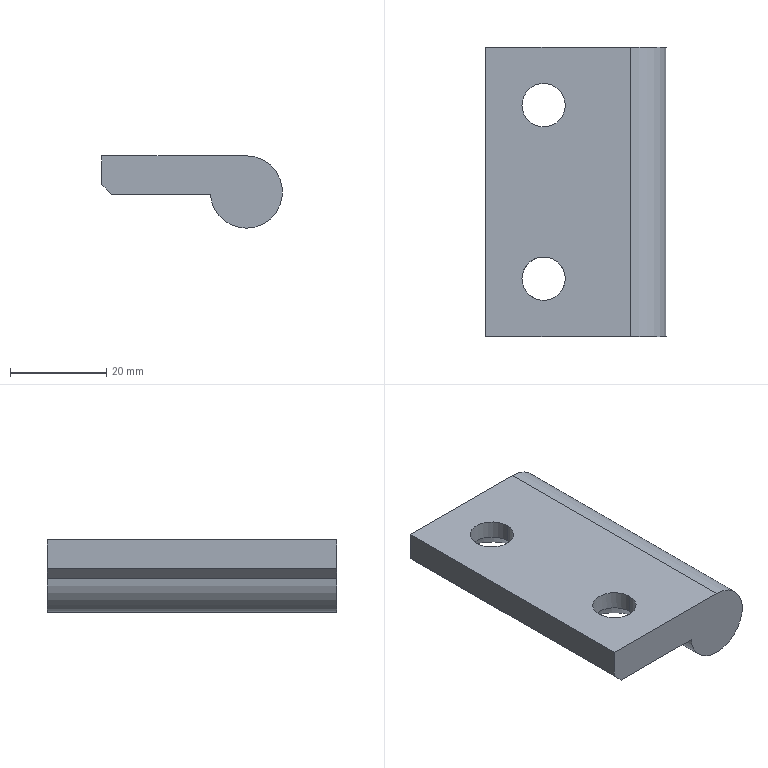Part | SolidWorks | features BaseBody 1 | 1 solid | 16 faces | box 37.5 x 60 x 15 mm | volume 20353 mm3 | cylinder 6 | plane 6 | cone 4 | commonest cylinder face diameters 9 x4 15 x2
STEP:
#1=CARTESIAN_POINT('',(0.,60.,-7.5));
#2=VERTEX_POINT('',#1);
#3=CARTESIAN_POINT('',(-7.483,60.,-0.5));
#4=VERTEX_POINT('',#3);
#5=CARTESIAN_POINT('',(0.,60.,0.));
#6=DIRECTION('',(0.,1.,0.));
#7=DIRECTION('',(0.,0.,-1.));
#8=AXIS2_PLACEMENT_3D('',#5,#6,#7);
#9=CIRCLE('',#8,7.5);
#10=EDGE_CURVE('',#2,#4,#9,.T.);
#11=ORIENTED_EDGE('',*,*,#10,.F.);
#12=CARTESIAN_POINT('',(0.,0.,-7.5));
#13=VERTEX_POINT('',#12);
#14=CARTESIAN_POINT('',(0.,60.,-7.5));
#15=DIRECTION('',(0.,-1.,0.));
#16=VECTOR('',#15,1000.);
#17=LINE('',#14,#16);
#18=EDGE_CURVE('',#2,#13,#17,.T.);
#19=ORIENTED_EDGE('',*,*,#18,.T.);
#20=CARTESIAN_POINT('',(-7.483,0.,-0.5));
#21=VERTEX_POINT('',#20);
#22=CARTESIAN_POINT('',(0.,0.,0.));
#23=DIRECTION('',(0.,1.,0.));
#24=DIRECTION('',(0.,0.,-1.));
#25=AXIS2_PLACEMENT_3D('',#22,#23,#24);
#26=CIRCLE('',#25,7.5);
#27=EDGE_CURVE('',#13,#21,#26,.T.);
#28=ORIENTED_EDGE('',*,*,#27,.T.);
#29=CARTESIAN_POINT('',(-7.483,60.,-0.5));
#30=DIRECTION('',(0.,1.,0.));
#31=VECTOR('',#30,1000.);
#32=LINE('',#29,#31);
#33=EDGE_CURVE('',#21,#4,#32,.T.);
#34=ORIENTED_EDGE('',*,*,#33,.T.);
#35=EDGE_LOOP('',(#11,#19,#28,#34));
#36=FACE_OUTER_BOUND('',#35,.T.);
#37=CARTESIAN_POINT('',(0.,60.,0.));
#38=DIRECTION('',(0.,-1.,0.));
#39=DIRECTION('',(0.,0.,-1.));
#40=AXIS2_PLACEMENT_3D('',#37,#38,#39);
#41=CYLINDRICAL_SURFACE('',#40,7.5);
#42=ADVANCED_FACE('',(#36),#41,.T.);
#43=CARTESIAN_POINT('',(-13.5,48.,7.5));
#44=VERTEX_POINT('',#43);
#45=CARTESIAN_POINT('',(-22.5,48.,7.5));
#46=VERTEX_POINT('',#45);
#47=CARTESIAN_POINT('',(-18.,48.,7.5));
#48=DIRECTION('',(0.,0.,-1.));
#49=DIRECTION('',(-1.,0.,0.));
#50=AXIS2_PLACEMENT_3D('',#47,#48,#49);
#51=CIRCLE('',#50,4.5);
#52=EDGE_CURVE('',#44,#46,#51,.T.);
#53=ORIENTED_EDGE('',*,*,#52,.F.);
#54=CARTESIAN_POINT('',(-13.5,48.,3.65));
#55=VERTEX_POINT('',#54);
#56=CARTESIAN_POINT('',(-13.5,48.,-0.5));
#57=DIRECTION('',(0.,0.,-1.));
#58=VECTOR('',#57,1000.);
#59=LINE('',#56,#58);
#60=EDGE_CURVE('',#44,#55,#59,.T.);
#61=ORIENTED_EDGE('',*,*,#60,.T.);
#62=CARTESIAN_POINT('',(-22.5,48.,3.65));
#63=VERTEX_POINT('',#62);
#64=CARTESIAN_POINT('',(-18.,48.,3.65));
#65=DIRECTION('',(0.,0.,1.));
#66=DIRECTION('',(-1.,0.,0.));
#67=AXIS2_PLACEMENT_3D('',#64,#65,#66);
#68=CIRCLE('',#67,4.5);
#69=EDGE_CURVE('',#63,#55,#68,.T.);
#70=ORIENTED_EDGE('',*,*,#69,.F.);
#71=CARTESIAN_POINT('',(-22.5,48.,-0.5));
#72=DIRECTION('',(0.,0.,-1.));
#73=VECTOR('',#72,1000.);
#74=LINE('',#71,#73);
#75=EDGE_CURVE('',#46,#63,#74,.T.);
#76=ORIENTED_EDGE('',*,*,#75,.F.);
#77=EDGE_LOOP('',(#53,#61,#70,#76));
#78=FACE_OUTER_BOUND('',#77,.T.);
#79=CARTESIAN_POINT('',(-18.,48.,-0.5));
#80=DIRECTION('',(0.,0.,-1.));
#81=DIRECTION('',(-1.,0.,0.));
#82=AXIS2_PLACEMENT_3D('',#79,#80,#81);
#83=CYLINDRICAL_SURFACE('',#82,4.5);
#84=ADVANCED_FACE('',(#78),#83,.F.);
#85=CARTESIAN_POINT('',(-13.5,12.,7.5));
#86=VERTEX_POINT('',#85);
#87=CARTESIAN_POINT('',(-22.5,12.,7.5));
#88=VERTEX_POINT('',#87);
#89=CARTESIAN_POINT('',(-18.,12.,7.5));
#90=DIRECTION('',(0.,0.,-1.));
#91=DIRECTION('',(-1.,0.,0.));
#92=AXIS2_PLACEMENT_3D('',#89,#90,#91);
#93=CIRCLE('',#92,4.5);
#94=EDGE_CURVE('',#86,#88,#93,.T.);
#95=ORIENTED_EDGE('',*,*,#94,.F.);
#96=CARTESIAN_POINT('',(-13.5,12.,3.65));
#97=VERTEX_POINT('',#96);
#98=CARTESIAN_POINT('',(-13.5,12.,-0.5));
#99=DIRECTION('',(0.,0.,-1.));
#100=VECTOR('',#99,1000.);
#101=LINE('',#98,#100);
#102=EDGE_CURVE('',#86,#97,#101,.T.);
#103=ORIENTED_EDGE('',*,*,#102,.T.);
#104=CARTESIAN_POINT('',(-18.,7.5,3.65));
#105=VERTEX_POINT('',#104);
#106=CARTESIAN_POINT('',(-18.,12.,3.65));
#107=DIRECTION('',(0.,0.,1.));
#108=DIRECTION('',(-1.,0.,0.));
#109=AXIS2_PLACEMENT_3D('',#106,#107,#108);
#110=CIRCLE('',#109,4.5);
#111=EDGE_CURVE('',#105,#97,#110,.T.);
#112=ORIENTED_EDGE('',*,*,#111,.F.);
#113=CARTESIAN_POINT('',(-22.5,12.,3.65));
#114=VERTEX_POINT('',#113);
#115=CARTESIAN_POINT('',(-18.,12.,3.65));
#116=DIRECTION('',(0.,0.,1.));
#117=DIRECTION('',(-1.,0.,0.));
#118=AXIS2_PLACEMENT_3D('',#115,#116,#117);
#119=CIRCLE('',#118,4.5);
#120=EDGE_CURVE('',#114,#105,#119,.T.);
#121=ORIENTED_EDGE('',*,*,#120,.F.);
#122=CARTESIAN_POINT('',(-22.5,12.,-0.5));
#123=DIRECTION('',(0.,0.,-1.));
#124=VECTOR('',#123,1000.);
#125=LINE('',#122,#124);
#126=EDGE_CURVE('',#88,#114,#125,.T.);
#127=ORIENTED_EDGE('',*,*,#126,.F.);
#128=EDGE_LOOP('',(#95,#103,#112,#121,#127));
#129=FACE_OUTER_BOUND('',#128,.T.);
#130=CARTESIAN_POINT('',(-18.,12.,-0.5));
#131=DIRECTION('',(0.,0.,-1.));
#132=DIRECTION('',(-1.,0.,0.));
#133=AXIS2_PLACEMENT_3D('',#130,#131,#132);
#134=CYLINDRICAL_SURFACE('',#133,4.5);
#135=ADVANCED_FACE('',(#129),#134,.F.);
#136=ORIENTED_EDGE('',*,*,#69,.T.);
#137=CARTESIAN_POINT('',(-9.35,48.,-0.5));
#138=VERTEX_POINT('',#137);
#139=CARTESIAN_POINT('',(-9.35,48.,-0.5));
#140=DIRECTION('',(0.7071,0.,-0.7071));
#141=VECTOR('',#140,1000.);
#142=LINE('',#139,#141);
#143=EDGE_CURVE('',#55,#138,#142,.T.);
#144=ORIENTED_EDGE('',*,*,#143,.T.);
#145=CARTESIAN_POINT('',(-26.65,48.,-0.5));
#146=VERTEX_POINT('',#145);
#147=CARTESIAN_POINT('',(-18.,48.,-0.5));
#148=DIRECTION('',(0.,0.,-1.));
#149=DIRECTION('',(0.,1.,0.));
#150=AXIS2_PLACEMENT_3D('',#147,#148,#149);
#151=CIRCLE('',#150,8.65);
#152=EDGE_CURVE('',#138,#146,#151,.T.);
#153=ORIENTED_EDGE('',*,*,#152,.T.);
#154=CARTESIAN_POINT('',(-26.65,48.,-0.5));
#155=DIRECTION('',(-0.7071,0.,-0.7071));
#156=VECTOR('',#155,1000.);
#157=LINE('',#154,#156);
#158=EDGE_CURVE('',#63,#146,#157,.T.);
#159=ORIENTED_EDGE('',*,*,#158,.F.);
#160=EDGE_LOOP('',(#136,#144,#153,#159));
#161=FACE_OUTER_BOUND('',#160,.T.);
#162=CARTESIAN_POINT('',(-18.,48.,-0.5));
#163=DIRECTION('',(0.,0.,-1.));
#164=DIRECTION('',(-1.,0.,0.));
#165=AXIS2_PLACEMENT_3D('',#162,#163,#164);
#166=CONICAL_SURFACE('',#165,8.65,0.7854);
#167=ADVANCED_FACE('',(#161),#166,.F.);
#168=CARTESIAN_POINT('',(-18.,16.5,3.65));
#169=VERTEX_POINT('',#168);
#170=CARTESIAN_POINT('',(-18.,12.,3.65));
#171=DIRECTION('',(0.,0.,1.));
#172=DIRECTION('',(-1.,0.,0.));
#173=AXIS2_PLACEMENT_3D('',#170,#171,#172);
#174=CIRCLE('',#173,4.5);
#175=EDGE_CURVE('',#169,#114,#174,.T.);
#176=ORIENTED_EDGE('',*,*,#175,.T.);
#177=ORIENTED_EDGE('',*,*,#120,.T.);
#178=CARTESIAN_POINT('',(-18.,3.35,-0.5));
#179=VERTEX_POINT('',#178);
#180=CARTESIAN_POINT('',(-18.,3.35,-0.5));
#181=DIRECTION('',(0.,-0.7071,-0.7071));
#182=VECTOR('',#181,1000.);
#183=LINE('',#180,#182);
#184=EDGE_CURVE('',#105,#179,#183,.T.);
#185=ORIENTED_EDGE('',*,*,#184,.T.);
#186=CARTESIAN_POINT('',(-18.,20.65,-0.5));
#187=VERTEX_POINT('',#186);
#188=CARTESIAN_POINT('',(-18.,12.,-0.5));
#189=DIRECTION('',(0.,0.,-1.));
#190=DIRECTION('',(0.,1.,0.));
#191=AXIS2_PLACEMENT_3D('',#188,#189,#190);
#192=CIRCLE('',#191,8.65);
#193=EDGE_CURVE('',#179,#187,#192,.T.);
#194=ORIENTED_EDGE('',*,*,#193,.T.);
#195=CARTESIAN_POINT('',(-18.,20.65,-0.5));
#196=DIRECTION('',(0.,0.7071,-0.7071));
#197=VECTOR('',#196,1000.);
#198=LINE('',#195,#197);
#199=EDGE_CURVE('',#169,#187,#198,.T.);
#200=ORIENTED_EDGE('',*,*,#199,.F.);
#201=EDGE_LOOP('',(#176,#177,#185,#194,#200));
#202=FACE_OUTER_BOUND('',#201,.T.);
#203=CARTESIAN_POINT('',(-18.,12.,-0.5));
#204=DIRECTION('',(0.,0.,-1.));
#205=DIRECTION('',(0.,1.,0.));
#206=AXIS2_PLACEMENT_3D('',#203,#204,#205);
#207=CONICAL_SURFACE('',#206,8.65,0.7854);
#208=ADVANCED_FACE('',(#202),#207,.F.);
#209=CARTESIAN_POINT('',(0.,60.,7.5));
#210=VERTEX_POINT('',#209);
#211=CARTESIAN_POINT('',(-30.,60.,7.5));
#212=VERTEX_POINT('',#211);
#213=CARTESIAN_POINT('',(0.,60.,7.5));
#214=DIRECTION('',(-1.,0.,0.));
#215=VECTOR('',#214,1000.);
#216=LINE('',#213,#215);
#217=EDGE_CURVE('',#210,#212,#216,.T.);
#218=ORIENTED_EDGE('',*,*,#217,.T.);
#219=CARTESIAN_POINT('',(-30.,0.,7.5));
#220=VERTEX_POINT('',#219);
#221=CARTESIAN_POINT('',(-30.,60.,7.5));
#222=DIRECTION('',(0.,-1.,0.));
#223=VECTOR('',#222,1000.);
#224=LINE('',#221,#223);
#225=EDGE_CURVE('',#212,#220,#224,.T.);
#226=ORIENTED_EDGE('',*,*,#225,.T.);
#227=CARTESIAN_POINT('',(0.,0.,7.5));
#228=VERTEX_POINT('',#227);
#229=CARTESIAN_POINT('',(0.,0.,7.5));
#230=DIRECTION('',(1.,0.,0.));
#231=VECTOR('',#230,1000.);
#232=LINE('',#229,#231);
#233=EDGE_CURVE('',#220,#228,#232,.T.);
#234=ORIENTED_EDGE('',*,*,#233,.T.);
#235=CARTESIAN_POINT('',(0.,60.,7.5));
#236=DIRECTION('',(0.,1.,0.));
#237=VECTOR('',#236,1000.);
#238=LINE('',#235,#237);
#239=EDGE_CURVE('',#228,#210,#238,.T.);
#240=ORIENTED_EDGE('',*,*,#239,.T.);
#241=EDGE_LOOP('',(#218,#226,#234,#240));
#242=FACE_OUTER_BOUND('',#241,.T.);
#243=CARTESIAN_POINT('',(-18.,48.,7.5));
#244=DIRECTION('',(0.,0.,-1.));
#245=DIRECTION('',(-1.,0.,0.));
#246=AXIS2_PLACEMENT_3D('',#243,#244,#245);
#247=CIRCLE('',#246,4.5);
#248=EDGE_CURVE('',#46,#44,#247,.T.);
#249=ORIENTED_EDGE('',*,*,#248,.T.);
#250=ORIENTED_EDGE('',*,*,#52,.T.);
#251=EDGE_LOOP('',(#249,#250));
#252=FACE_BOUND('',#251,.T.);
#253=CARTESIAN_POINT('',(-18.,12.,7.5));
#254=DIRECTION('',(0.,0.,-1.));
#255=DIRECTION('',(-1.,0.,0.));
#256=AXIS2_PLACEMENT_3D('',#253,#254,#255);
#257=CIRCLE('',#256,4.5);
#258=EDGE_CURVE('',#88,#86,#257,.T.);
#259=ORIENTED_EDGE('',*,*,#258,.T.);
#260=ORIENTED_EDGE('',*,*,#94,.T.);
#261=EDGE_LOOP('',(#259,#260));
#262=FACE_BOUND('',#261,.T.);
#263=CARTESIAN_POINT('',(0.,60.,7.5));
#264=DIRECTION('',(0.,0.,1.));
#265=DIRECTION('',(1.,0.,0.));
#266=AXIS2_PLACEMENT_3D('',#263,#264,#265);
#267=PLANE('',#266);
#268=ADVANCED_FACE('',(#242,#252,#262),#267,.T.);
#269=CARTESIAN_POINT('',(-30.,0.,1.5));
#270=VERTEX_POINT('',#269);
#271=CARTESIAN_POINT('',(-30.,0.,0.));
#272=DIRECTION('',(0.,0.,1.));
#273=VECTOR('',#272,1000.);
#274=LINE('',#271,#273);
#275=EDGE_CURVE('',#270,#220,#274,.T.);
#276=ORIENTED_EDGE('',*,*,#275,.T.);
#277=ORIENTED_EDGE('',*,*,#225,.F.);
#278=CARTESIAN_POINT('',(-30.,60.,1.5));
#279=VERTEX_POINT('',#278);
#280=CARTESIAN_POINT('',(-30.,60.,0.));
#281=DIRECTION('',(0.,0.,-1.));
#282=VECTOR('',#281,1000.);
#283=LINE('',#280,#282);
#284=EDGE_CURVE('',#212,#279,#283,.T.);
#285=ORIENTED_EDGE('',*,*,#284,.T.);
#286=CARTESIAN_POINT('',(-30.,60.,1.5));
#287=DIRECTION('',(0.,-1.,0.));
#288=VECTOR('',#287,1000.);
#289=LINE('',#286,#288);
#290=EDGE_CURVE('',#279,#270,#289,.T.);
#291=ORIENTED_EDGE('',*,*,#290,.T.);
#292=EDGE_LOOP('',(#276,#277,#285,#291));
#293=FACE_OUTER_BOUND('',#292,.T.);
#294=CARTESIAN_POINT('',(-30.,60.,0.));
#295=DIRECTION('',(-1.,0.,0.));
#296=DIRECTION('',(0.,0.,1.));
#297=AXIS2_PLACEMENT_3D('',#294,#295,#296);
#298=PLANE('',#297);
#299=ADVANCED_FACE('',(#293),#298,.T.);
#300=ORIENTED_EDGE('',*,*,#217,.F.);
#301=CARTESIAN_POINT('',(0.,60.,0.));
#302=DIRECTION('',(0.,1.,0.));
#303=DIRECTION('',(0.,0.,-1.));
#304=AXIS2_PLACEMENT_3D('',#301,#302,#303);
#305=CIRCLE('',#304,7.5);
#306=EDGE_CURVE('',#210,#2,#305,.T.);
#307=ORIENTED_EDGE('',*,*,#306,.T.);
#308=ORIENTED_EDGE('',*,*,#10,.T.);
#309=CARTESIAN_POINT('',(-28.,60.,-0.5));
#310=VERTEX_POINT('',#309);
#311=CARTESIAN_POINT('',(0.,60.,-0.5));
#312=DIRECTION('',(-1.,0.,0.));
#313=VECTOR('',#312,1000.);
#314=LINE('',#311,#313);
#315=EDGE_CURVE('',#4,#310,#314,.T.);
#316=ORIENTED_EDGE('',*,*,#315,.T.);
#317=CARTESIAN_POINT('',(-28.,60.,-0.5));
#318=DIRECTION('',(-0.7071,0.,0.7071));
#319=VECTOR('',#318,1000.);
#320=LINE('',#317,#319);
#321=EDGE_CURVE('',#310,#279,#320,.T.);
#322=ORIENTED_EDGE('',*,*,#321,.T.);
#323=ORIENTED_EDGE('',*,*,#284,.F.);
#324=EDGE_LOOP('',(#300,#307,#308,#316,#322,#323));
#325=FACE_OUTER_BOUND('',#324,.T.);
#326=CARTESIAN_POINT('',(0.,60.,0.));
#327=DIRECTION('',(0.,1.,0.));
#328=DIRECTION('',(0.,0.,1.));
#329=AXIS2_PLACEMENT_3D('',#326,#327,#328);
#330=PLANE('',#329);
#331=ADVANCED_FACE('',(#325),#330,.T.);
#332=ORIENTED_EDGE('',*,*,#18,.F.);
#333=ORIENTED_EDGE('',*,*,#306,.F.);
#334=ORIENTED_EDGE('',*,*,#239,.F.);
#335=CARTESIAN_POINT('',(0.,0.,0.));
#336=DIRECTION('',(0.,1.,0.));
#337=DIRECTION('',(0.,0.,-1.));
#338=AXIS2_PLACEMENT_3D('',#335,#336,#337);
#339=CIRCLE('',#338,7.5);
#340=EDGE_CURVE('',#228,#13,#339,.T.);
#341=ORIENTED_EDGE('',*,*,#340,.T.);
#342=EDGE_LOOP('',(#332,#333,#334,#341));
#343=FACE_OUTER_BOUND('',#342,.T.);
#344=CARTESIAN_POINT('',(0.,60.,0.));
#345=DIRECTION('',(0.,-1.,0.));
#346=DIRECTION('',(0.,0.,-1.));
#347=AXIS2_PLACEMENT_3D('',#344,#345,#346);
#348=CYLINDRICAL_SURFACE('',#347,7.5);
#349=ADVANCED_FACE('',(#343),#348,.T.);
#350=CARTESIAN_POINT('',(-28.,0.,-0.5));
#351=VERTEX_POINT('',#350);
#352=CARTESIAN_POINT('',(-28.,0.,-0.5));
#353=DIRECTION('',(-0.7071,0.,0.7071));
#354=VECTOR('',#353,1000.);
#355=LINE('',#352,#354);
#356=EDGE_CURVE('',#351,#270,#355,.T.);
#357=ORIENTED_EDGE('',*,*,#356,.F.);
#358=CARTESIAN_POINT('',(0.,0.,-0.5));
#359=DIRECTION('',(-1.,0.,0.));
#360=VECTOR('',#359,1000.);
#361=LINE('',#358,#360);
#362=EDGE_CURVE('',#21,#351,#361,.T.);
#363=ORIENTED_EDGE('',*,*,#362,.F.);
#364=ORIENTED_EDGE('',*,*,#27,.F.);
#365=ORIENTED_EDGE('',*,*,#340,.F.);
#366=ORIENTED_EDGE('',*,*,#233,.F.);
#367=ORIENTED_EDGE('',*,*,#275,.F.);
#368=EDGE_LOOP('',(#357,#363,#364,#365,#366,#367));
#369=FACE_OUTER_BOUND('',#368,.T.);
#370=CARTESIAN_POINT('',(0.,0.,0.));
#371=DIRECTION('',(0.,1.,0.));
#372=DIRECTION('',(0.,0.,1.));
#373=AXIS2_PLACEMENT_3D('',#370,#371,#372);
#374=PLANE('',#373);
#375=ADVANCED_FACE('',(#369),#374,.F.);
#376=ORIENTED_EDGE('',*,*,#60,.F.);
#377=ORIENTED_EDGE('',*,*,#248,.F.);
#378=ORIENTED_EDGE('',*,*,#75,.T.);
#379=CARTESIAN_POINT('',(-18.,48.,3.65));
#380=DIRECTION('',(0.,0.,1.));
#381=DIRECTION('',(-1.,0.,0.));
#382=AXIS2_PLACEMENT_3D('',#379,#380,#381);
#383=CIRCLE('',#382,4.5);
#384=EDGE_CURVE('',#55,#63,#383,.T.);
#385=ORIENTED_EDGE('',*,*,#384,.F.);
#386=EDGE_LOOP('',(#376,#377,#378,#385));
#387=FACE_OUTER_BOUND('',#386,.T.);
#388=CARTESIAN_POINT('',(-18.,48.,-0.5));
#389=DIRECTION('',(0.,0.,-1.));
#390=DIRECTION('',(-1.,0.,0.));
#391=AXIS2_PLACEMENT_3D('',#388,#389,#390);
#392=CYLINDRICAL_SURFACE('',#391,4.5);
#393=ADVANCED_FACE('',(#387),#392,.F.);
#394=ORIENTED_EDGE('',*,*,#102,.F.);
#395=ORIENTED_EDGE('',*,*,#258,.F.);
#396=ORIENTED_EDGE('',*,*,#126,.T.);
#397=ORIENTED_EDGE('',*,*,#175,.F.);
#398=CARTESIAN_POINT('',(-18.,12.,3.65));
#399=DIRECTION('',(0.,0.,1.));
#400=DIRECTION('',(-1.,0.,0.));
#401=AXIS2_PLACEMENT_3D('',#398,#399,#400);
#402=CIRCLE('',#401,4.5);
#403=EDGE_CURVE('',#97,#169,#402,.T.);
#404=ORIENTED_EDGE('',*,*,#403,.F.);
#405=EDGE_LOOP('',(#394,#395,#396,#397,#404));
#406=FACE_OUTER_BOUND('',#405,.T.);
#407=CARTESIAN_POINT('',(-18.,12.,-0.5));
#408=DIRECTION('',(0.,0.,-1.));
#409=DIRECTION('',(-1.,0.,0.));
#410=AXIS2_PLACEMENT_3D('',#407,#408,#409);
#411=CYLINDRICAL_SURFACE('',#410,4.5);
#412=ADVANCED_FACE('',(#406),#411,.F.);
#413=ORIENTED_EDGE('',*,*,#356,.T.);
#414=ORIENTED_EDGE('',*,*,#290,.F.);
#415=ORIENTED_EDGE('',*,*,#321,.F.);
#416=CARTESIAN_POINT('',(-28.,60.,-0.5));
#417=DIRECTION('',(0.,-1.,0.));
#418=VECTOR('',#417,1000.);
#419=LINE('',#416,#418);
#420=EDGE_CURVE('',#310,#351,#419,.T.);
#421=ORIENTED_EDGE('',*,*,#420,.T.);
#422=EDGE_LOOP('',(#413,#414,#415,#421));
#423=FACE_OUTER_BOUND('',#422,.T.);
#424=CARTESIAN_POINT('',(-30.,60.,1.5));
#425=DIRECTION('',(-0.7071,0.,-0.7071));
#426=DIRECTION('',(-0.7071,0.,0.7071));
#427=AXIS2_PLACEMENT_3D('',#424,#425,#426);
#428=PLANE('',#427);
#429=ADVANCED_FACE('',(#423),#428,.T.);
#430=ORIENTED_EDGE('',*,*,#420,.F.);
#431=ORIENTED_EDGE('',*,*,#315,.F.);
#432=ORIENTED_EDGE('',*,*,#33,.F.);
#433=ORIENTED_EDGE('',*,*,#362,.T.);
#434=EDGE_LOOP('',(#430,#431,#432,#433));
#435=FACE_OUTER_BOUND('',#434,.T.);
#436=CARTESIAN_POINT('',(-18.,48.,-0.5));
#437=DIRECTION('',(0.,0.,-1.));
#438=DIRECTION('',(0.,1.,0.));
#439=AXIS2_PLACEMENT_3D('',#436,#437,#438);
#440=CIRCLE('',#439,8.65);
#441=EDGE_CURVE('',#146,#138,#440,.T.);
#442=ORIENTED_EDGE('',*,*,#441,.F.);
#443=ORIENTED_EDGE('',*,*,#152,.F.);
#444=EDGE_LOOP('',(#442,#443));
#445=FACE_BOUND('',#444,.T.);
#446=CARTESIAN_POINT('',(-18.,12.,-0.5));
#447=DIRECTION('',(0.,0.,-1.));
#448=DIRECTION('',(0.,1.,0.));
#449=AXIS2_PLACEMENT_3D('',#446,#447,#448);
#450=CIRCLE('',#449,8.65);
#451=EDGE_CURVE('',#187,#179,#450,.T.);
#452=ORIENTED_EDGE('',*,*,#451,.F.);
#453=ORIENTED_EDGE('',*,*,#193,.F.);
#454=EDGE_LOOP('',(#452,#453));
#455=FACE_BOUND('',#454,.T.);
#456=CARTESIAN_POINT('',(0.,60.,-0.5));
#457=DIRECTION('',(0.,0.,1.));
#458=DIRECTION('',(1.,0.,0.));
#459=AXIS2_PLACEMENT_3D('',#456,#457,#458);
#460=PLANE('',#459);
#461=ADVANCED_FACE('',(#435,#445,#455),#460,.F.);
#462=ORIENTED_EDGE('',*,*,#143,.F.);
#463=ORIENTED_EDGE('',*,*,#384,.T.);
#464=ORIENTED_EDGE('',*,*,#158,.T.);
#465=ORIENTED_EDGE('',*,*,#441,.T.);
#466=EDGE_LOOP('',(#462,#463,#464,#465));
#467=FACE_OUTER_BOUND('',#466,.T.);
#468=CARTESIAN_POINT('',(-18.,48.,-0.5));
#469=DIRECTION('',(0.,0.,-1.));
#470=DIRECTION('',(-1.,0.,0.));
#471=AXIS2_PLACEMENT_3D('',#468,#469,#470);
#472=CONICAL_SURFACE('',#471,8.65,0.7854);
#473=ADVANCED_FACE('',(#467),#472,.F.);
#474=ORIENTED_EDGE('',*,*,#184,.F.);
#475=ORIENTED_EDGE('',*,*,#111,.T.);
#476=ORIENTED_EDGE('',*,*,#403,.T.);
#477=ORIENTED_EDGE('',*,*,#199,.T.);
#478=ORIENTED_EDGE('',*,*,#451,.T.);
#479=EDGE_LOOP('',(#474,#475,#476,#477,#478));
#480=FACE_OUTER_BOUND('',#479,.T.);
#481=CARTESIAN_POINT('',(-18.,12.,-0.5));
#482=DIRECTION('',(0.,0.,-1.));
#483=DIRECTION('',(0.,1.,0.));
#484=AXIS2_PLACEMENT_3D('',#481,#482,#483);
#485=CONICAL_SURFACE('',#484,8.65,0.7854);
#486=ADVANCED_FACE('',(#480),#485,.F.);
#487=CLOSED_SHELL('',(#42,#84,#135,#167,#208,#268,#299,#331,#349,#375,#393,#412,#429,#461,#473,#486));
#488=MANIFOLD_SOLID_BREP('',#487);
#489=CARTESIAN_POINT('',(0.,0.,0.));
#490=DIRECTION('',(0.,0.,1.));
#491=DIRECTION('',(1.,0.,0.));
#492=AXIS2_PLACEMENT_3D('',#489,#490,#491);
#493=(LENGTH_UNIT()NAMED_UNIT(*)SI_UNIT(.MILLI.,.METRE.));
#494=UNCERTAINTY_MEASURE_WITH_UNIT(LENGTH_MEASURE(0.00001),#493,'','');
#495=(NAMED_UNIT(*)PLANE_ANGLE_UNIT()SI_UNIT($,.RADIAN.));
#496=(NAMED_UNIT(*)SI_UNIT($,.STERADIAN.)SOLID_ANGLE_UNIT());
#497=(GEOMETRIC_REPRESENTATION_CONTEXT(3)GLOBAL_UNCERTAINTY_ASSIGNED_CONTEXT((#494))GLOBAL_UNIT_ASSIGNED_CONTEXT((#493,#495,#496))REPRESENTATION_CONTEXT('',''));
#498=ADVANCED_BREP_SHAPE_REPRESENTATION('',(#488,#492),#497);